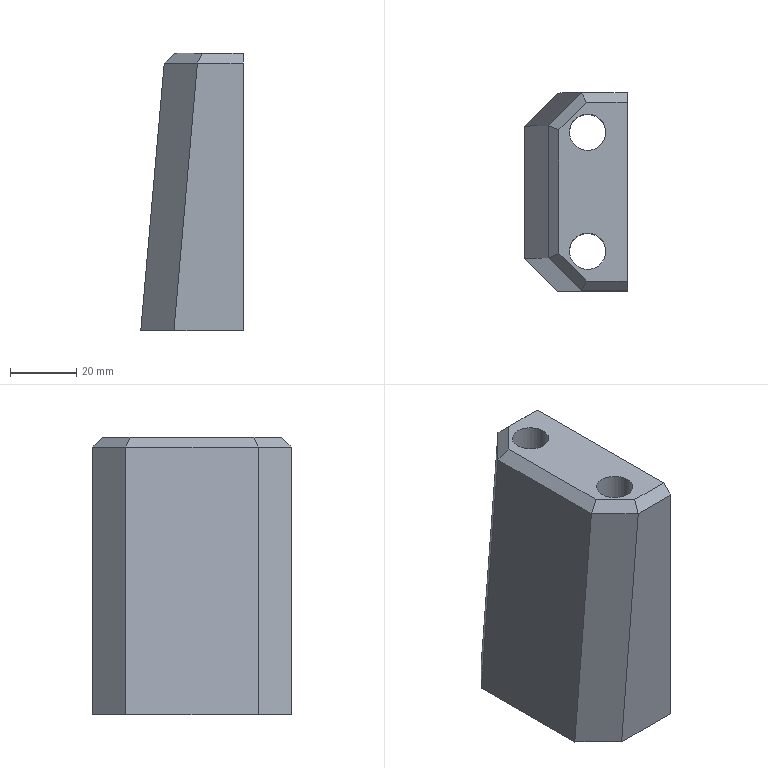Part | STEP file | P011002NF03-000 | 1 solid | 29 faces | box 31 x 60 x 84 mm | volume 108643 mm3 | plane 13 | cylinder 7 | spline 6 | cone 3 | commonest cylinder face diameters 11 x2 17 x2 8.5 x1 9.967 x1 10 x1